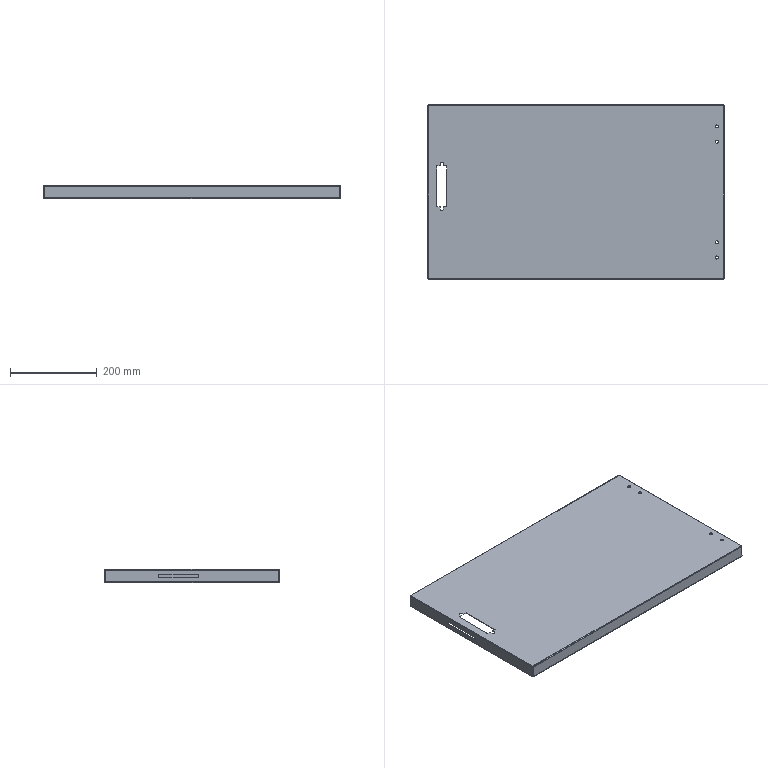Part | 1 solid | 95 faces | box 683 x 402 x 30 mm | volume 424841 mm3 | plane 50 | cylinder 29 | spline 16 | commonest cylinder face diameters 7 x13 1.473 x8 3.873 x8